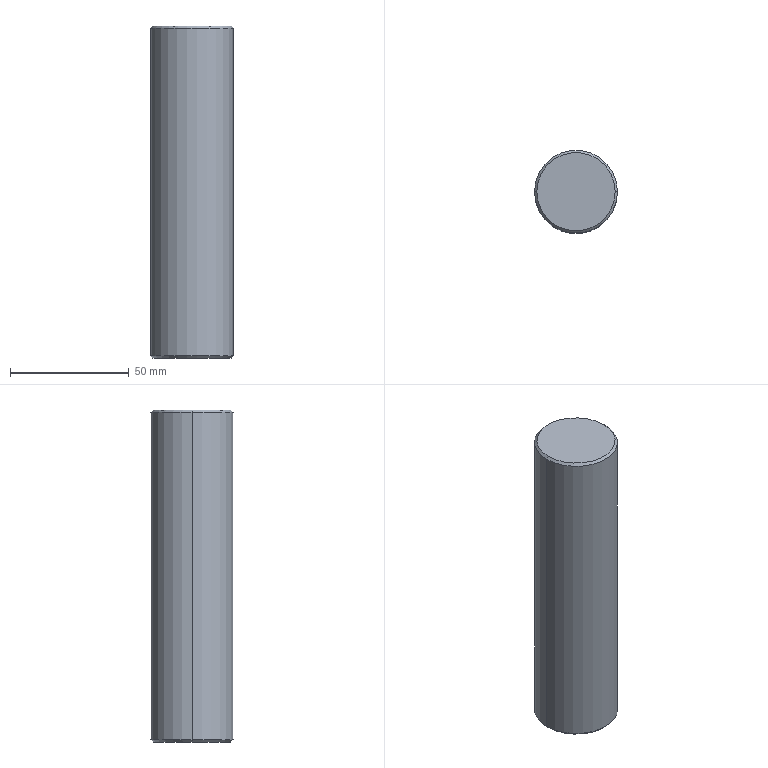Part | Creo | 1 solid | 16 faces | box 35 x 35 x 140 mm | volume 133063 mm3 | cone 8 | cylinder 6 | plane 2 | commonest cylinder face diameters 8.46 x2 10 x2 35 x2
STEP:
#1=CARTESIAN_POINT('',(0.,0.,0.));
#2=DIRECTION('',(0.,0.,1.));
#3=DIRECTION('',(1.,0.,0.));
#4=AXIS2_PLACEMENT_3D('',#1,#2,#3);
#5=CARTESIAN_POINT('',(16.5,43.,-260.5));
#6=VERTEX_POINT('',#5);
#7=CARTESIAN_POINT('',(-16.5,43.,-260.5));
#8=VERTEX_POINT('',#7);
#9=CARTESIAN_POINT('',(0.,43.,-260.5));
#10=DIRECTION('',(0.,0.,-1.));
#11=DIRECTION('',(1.,0.,0.));
#12=AXIS2_PLACEMENT_3D('',#9,#10,#11);
#13=CIRCLE('',#12,16.5);
#14=EDGE_CURVE('',#6,#8,#13,.T.);
#15=ORIENTED_EDGE('',*,*,#14,.F.);
#16=CARTESIAN_POINT('',(0.,43.,-260.5));
#17=DIRECTION('',(0.,0.,-1.));
#18=DIRECTION('',(-1.,0.,0.));
#19=AXIS2_PLACEMENT_3D('',#16,#17,#18);
#20=CIRCLE('',#19,16.5);
#21=EDGE_CURVE('',#8,#6,#20,.T.);
#22=ORIENTED_EDGE('',*,*,#21,.F.);
#23=EDGE_LOOP('',(#15,#22));
#24=FACE_OUTER_BOUND('',#23,.F.);
#25=CARTESIAN_POINT('',(-5.,43.,-260.5));
#26=VERTEX_POINT('',#25);
#27=CARTESIAN_POINT('',(5.,43.,-260.5));
#28=VERTEX_POINT('',#27);
#29=CARTESIAN_POINT('',(0.,43.,-260.5));
#30=DIRECTION('',(0.,0.,1.));
#31=DIRECTION('',(-1.,0.,0.));
#32=AXIS2_PLACEMENT_3D('',#29,#30,#31);
#33=CIRCLE('',#32,5.);
#34=EDGE_CURVE('',#26,#28,#33,.T.);
#35=ORIENTED_EDGE('',*,*,#34,.F.);
#36=CARTESIAN_POINT('',(0.,43.,-260.5));
#37=DIRECTION('',(0.,0.,1.));
#38=DIRECTION('',(1.,0.,0.));
#39=AXIS2_PLACEMENT_3D('',#36,#37,#38);
#40=CIRCLE('',#39,5.);
#41=EDGE_CURVE('',#28,#26,#40,.T.);
#42=ORIENTED_EDGE('',*,*,#41,.F.);
#43=EDGE_LOOP('',(#35,#42));
#44=FACE_BOUND('',#43,.F.);
#45=CARTESIAN_POINT('',(0.,43.,-260.5));
#46=DIRECTION('',(0.,0.,1.));
#47=DIRECTION('',(1.,0.,0.));
#48=AXIS2_PLACEMENT_3D('',#45,#46,#47);
#49=PLANE('',#48);
#50=ADVANCED_FACE('',(#24,#44),#49,.F.);
#51=ORIENTED_EDGE('',*,*,#14,.T.);
#52=CARTESIAN_POINT('',(-17.5,43.,-259.5));
#53=VERTEX_POINT('',#52);
#54=CARTESIAN_POINT('',(-16.5,43.,-260.5));
#55=DIRECTION('',(-0.7071,0.,0.7071));
#56=VECTOR('',#55,1.414);
#57=LINE('',#54,#56);
#58=EDGE_CURVE('',#8,#53,#57,.T.);
#59=ORIENTED_EDGE('',*,*,#58,.T.);
#60=CARTESIAN_POINT('',(17.5,43.,-259.5));
#61=VERTEX_POINT('',#60);
#62=CARTESIAN_POINT('',(0.,43.,-259.5));
#63=DIRECTION('',(0.,0.,-1.));
#64=DIRECTION('',(1.,0.,0.));
#65=AXIS2_PLACEMENT_3D('',#62,#63,#64);
#66=CIRCLE('',#65,17.5);
#67=EDGE_CURVE('',#61,#53,#66,.T.);
#68=ORIENTED_EDGE('',*,*,#67,.F.);
#69=CARTESIAN_POINT('',(16.5,43.,-260.5));
#70=DIRECTION('',(0.7071,0.,0.7071));
#71=VECTOR('',#70,1.414);
#72=LINE('',#69,#71);
#73=EDGE_CURVE('',#6,#61,#72,.T.);
#74=ORIENTED_EDGE('',*,*,#73,.F.);
#75=EDGE_LOOP('',(#51,#59,#68,#74));
#76=FACE_OUTER_BOUND('',#75,.F.);
#77=CARTESIAN_POINT('',(0.,43.,-260.));
#78=DIRECTION('',(0.,0.,1.));
#79=DIRECTION('',(1.,0.,0.));
#80=AXIS2_PLACEMENT_3D('',#77,#78,#79);
#81=CONICAL_SURFACE('',#80,17.,45.);
#82=ADVANCED_FACE('',(#76),#81,.T.);
#83=ORIENTED_EDGE('',*,*,#21,.T.);
#84=ORIENTED_EDGE('',*,*,#73,.T.);
#85=CARTESIAN_POINT('',(0.,43.,-259.5));
#86=DIRECTION('',(0.,0.,-1.));
#87=DIRECTION('',(-1.,0.,0.));
#88=AXIS2_PLACEMENT_3D('',#85,#86,#87);
#89=CIRCLE('',#88,17.5);
#90=EDGE_CURVE('',#53,#61,#89,.T.);
#91=ORIENTED_EDGE('',*,*,#90,.F.);
#92=ORIENTED_EDGE('',*,*,#58,.F.);
#93=EDGE_LOOP('',(#83,#84,#91,#92));
#94=FACE_OUTER_BOUND('',#93,.F.);
#95=CARTESIAN_POINT('',(0.,43.,-260.));
#96=DIRECTION('',(0.,0.,1.));
#97=DIRECTION('',(1.,0.,0.));
#98=AXIS2_PLACEMENT_3D('',#95,#96,#97);
#99=CONICAL_SURFACE('',#98,17.,45.);
#100=ADVANCED_FACE('',(#94),#99,.T.);
#101=ORIENTED_EDGE('',*,*,#90,.T.);
#102=CARTESIAN_POINT('',(17.5,43.,-121.5));
#103=VERTEX_POINT('',#102);
#104=CARTESIAN_POINT('',(17.5,43.,-121.5));
#105=DIRECTION('',(0.,0.,-1.));
#106=VECTOR('',#105,138.);
#107=LINE('',#104,#106);
#108=EDGE_CURVE('',#103,#61,#107,.T.);
#109=ORIENTED_EDGE('',*,*,#108,.F.);
#110=CARTESIAN_POINT('',(-17.5,43.,-121.5));
#111=VERTEX_POINT('',#110);
#112=CARTESIAN_POINT('',(0.,43.,-121.5));
#113=DIRECTION('',(0.,0.,1.));
#114=DIRECTION('',(1.,0.,0.));
#115=AXIS2_PLACEMENT_3D('',#112,#113,#114);
#116=CIRCLE('',#115,17.5);
#117=EDGE_CURVE('',#103,#111,#116,.T.);
#118=ORIENTED_EDGE('',*,*,#117,.T.);
#119=CARTESIAN_POINT('',(-17.5,43.,-121.5));
#120=DIRECTION('',(0.,0.,-1.));
#121=VECTOR('',#120,138.);
#122=LINE('',#119,#121);
#123=EDGE_CURVE('',#111,#53,#122,.T.);
#124=ORIENTED_EDGE('',*,*,#123,.T.);
#125=EDGE_LOOP('',(#101,#109,#118,#124));
#126=FACE_OUTER_BOUND('',#125,.F.);
#127=CARTESIAN_POINT('',(0.,43.,-120.5));
#128=DIRECTION('',(0.,0.,-1.));
#129=DIRECTION('',(-1.,0.,0.));
#130=AXIS2_PLACEMENT_3D('',#127,#128,#129);
#131=CYLINDRICAL_SURFACE('',#130,17.5);
#132=ADVANCED_FACE('',(#126),#131,.T.);
#133=ORIENTED_EDGE('',*,*,#67,.T.);
#134=ORIENTED_EDGE('',*,*,#123,.F.);
#135=CARTESIAN_POINT('',(0.,43.,-121.5));
#136=DIRECTION('',(0.,0.,1.));
#137=DIRECTION('',(-1.,0.,0.));
#138=AXIS2_PLACEMENT_3D('',#135,#136,#137);
#139=CIRCLE('',#138,17.5);
#140=EDGE_CURVE('',#111,#103,#139,.T.);
#141=ORIENTED_EDGE('',*,*,#140,.T.);
#142=ORIENTED_EDGE('',*,*,#108,.T.);
#143=EDGE_LOOP('',(#133,#134,#141,#142));
#144=FACE_OUTER_BOUND('',#143,.F.);
#145=CARTESIAN_POINT('',(0.,43.,-120.5));
#146=DIRECTION('',(0.,0.,-1.));
#147=DIRECTION('',(-1.,0.,0.));
#148=AXIS2_PLACEMENT_3D('',#145,#146,#147);
#149=CYLINDRICAL_SURFACE('',#148,17.5);
#150=ADVANCED_FACE('',(#144),#149,.T.);
#151=ORIENTED_EDGE('',*,*,#140,.F.);
#152=CARTESIAN_POINT('',(-16.5,43.,-120.5));
#153=VERTEX_POINT('',#152);
#154=CARTESIAN_POINT('',(-16.5,43.,-120.5));
#155=DIRECTION('',(-0.7071,0.,-0.7071));
#156=VECTOR('',#155,1.414);
#157=LINE('',#154,#156);
#158=EDGE_CURVE('',#153,#111,#157,.T.);
#159=ORIENTED_EDGE('',*,*,#158,.F.);
#160=CARTESIAN_POINT('',(16.5,43.,-120.5));
#161=VERTEX_POINT('',#160);
#162=CARTESIAN_POINT('',(0.,43.,-120.5));
#163=DIRECTION('',(0.,0.,1.));
#164=DIRECTION('',(-1.,0.,0.));
#165=AXIS2_PLACEMENT_3D('',#162,#163,#164);
#166=CIRCLE('',#165,16.5);
#167=EDGE_CURVE('',#153,#161,#166,.T.);
#168=ORIENTED_EDGE('',*,*,#167,.T.);
#169=CARTESIAN_POINT('',(16.5,43.,-120.5));
#170=DIRECTION('',(0.7071,0.,-0.7071));
#171=VECTOR('',#170,1.414);
#172=LINE('',#169,#171);
#173=EDGE_CURVE('',#161,#103,#172,.T.);
#174=ORIENTED_EDGE('',*,*,#173,.T.);
#175=EDGE_LOOP('',(#151,#159,#168,#174));
#176=FACE_OUTER_BOUND('',#175,.F.);
#177=CARTESIAN_POINT('',(0.,43.,-121.));
#178=DIRECTION('',(0.,0.,-1.));
#179=DIRECTION('',(-1.,0.,0.));
#180=AXIS2_PLACEMENT_3D('',#177,#178,#179);
#181=CONICAL_SURFACE('',#180,17.,45.);
#182=ADVANCED_FACE('',(#176),#181,.T.);
#183=ORIENTED_EDGE('',*,*,#117,.F.);
#184=ORIENTED_EDGE('',*,*,#173,.F.);
#185=CARTESIAN_POINT('',(0.,43.,-120.5));
#186=DIRECTION('',(0.,0.,1.));
#187=DIRECTION('',(1.,0.,0.));
#188=AXIS2_PLACEMENT_3D('',#185,#186,#187);
#189=CIRCLE('',#188,16.5);
#190=EDGE_CURVE('',#161,#153,#189,.T.);
#191=ORIENTED_EDGE('',*,*,#190,.T.);
#192=ORIENTED_EDGE('',*,*,#158,.T.);
#193=EDGE_LOOP('',(#183,#184,#191,#192));
#194=FACE_OUTER_BOUND('',#193,.F.);
#195=CARTESIAN_POINT('',(0.,43.,-121.));
#196=DIRECTION('',(0.,0.,-1.));
#197=DIRECTION('',(-1.,0.,0.));
#198=AXIS2_PLACEMENT_3D('',#195,#196,#197);
#199=CONICAL_SURFACE('',#198,17.,45.);
#200=ADVANCED_FACE('',(#194),#199,.T.);
#201=ORIENTED_EDGE('',*,*,#190,.F.);
#202=ORIENTED_EDGE('',*,*,#167,.F.);
#203=EDGE_LOOP('',(#201,#202));
#204=FACE_OUTER_BOUND('',#203,.F.);
#205=CARTESIAN_POINT('',(0.,43.,-120.5));
#206=DIRECTION('',(0.,0.,1.));
#207=DIRECTION('',(1.,0.,0.));
#208=AXIS2_PLACEMENT_3D('',#205,#206,#207);
#209=PLANE('',#208);
#210=ADVANCED_FACE('',(#204),#209,.T.);
#211=CARTESIAN_POINT('',(5.,43.,-244.5));
#212=VERTEX_POINT('',#211);
#213=CARTESIAN_POINT('',(-5.,43.,-244.5));
#214=VERTEX_POINT('',#213);
#215=CARTESIAN_POINT('',(0.,43.,-244.5));
#216=DIRECTION('',(0.,0.,-1.));
#217=DIRECTION('',(1.,0.,0.));
#218=AXIS2_PLACEMENT_3D('',#215,#216,#217);
#219=CIRCLE('',#218,5.);
#220=EDGE_CURVE('',#212,#214,#219,.T.);
#221=ORIENTED_EDGE('',*,*,#220,.T.);
#222=CARTESIAN_POINT('',(-5.,43.,-244.5));
#223=DIRECTION('',(0.,0.,-1.));
#224=VECTOR('',#223,16.);
#225=LINE('',#222,#224);
#226=EDGE_CURVE('',#214,#26,#225,.T.);
#227=ORIENTED_EDGE('',*,*,#226,.T.);
#228=ORIENTED_EDGE('',*,*,#34,.T.);
#229=CARTESIAN_POINT('',(5.,43.,-244.5));
#230=DIRECTION('',(0.,0.,-1.));
#231=VECTOR('',#230,16.);
#232=LINE('',#229,#231);
#233=EDGE_CURVE('',#212,#28,#232,.T.);
#234=ORIENTED_EDGE('',*,*,#233,.F.);
#235=EDGE_LOOP('',(#221,#227,#228,#234));
#236=FACE_OUTER_BOUND('',#235,.F.);
#237=CARTESIAN_POINT('',(0.,43.,-295.5));
#238=DIRECTION('',(0.,0.,-1.));
#239=DIRECTION('',(-1.,0.,0.));
#240=AXIS2_PLACEMENT_3D('',#237,#238,#239);
#241=CYLINDRICAL_SURFACE('',#240,5.);
#242=ADVANCED_FACE('',(#236),#241,.F.);
#243=CARTESIAN_POINT('',(-4.23,43.,-243.73));
#244=VERTEX_POINT('',#243);
#245=CARTESIAN_POINT('',(4.23,43.,-243.73));
#246=VERTEX_POINT('',#245);
#247=CARTESIAN_POINT('',(0.,43.,-243.73));
#248=DIRECTION('',(0.,0.,1.));
#249=DIRECTION('',(-1.,0.,0.));
#250=AXIS2_PLACEMENT_3D('',#247,#248,#249);
#251=CIRCLE('',#250,4.23);
#252=EDGE_CURVE('',#244,#246,#251,.T.);
#253=ORIENTED_EDGE('',*,*,#252,.F.);
#254=CARTESIAN_POINT('',(-4.23,43.,-243.73));
#255=DIRECTION('',(-0.7071,0.,-0.7071));
#256=VECTOR('',#255,1.089);
#257=LINE('',#254,#256);
#258=EDGE_CURVE('',#244,#214,#257,.T.);
#259=ORIENTED_EDGE('',*,*,#258,.T.);
#260=ORIENTED_EDGE('',*,*,#220,.F.);
#261=CARTESIAN_POINT('',(4.23,43.,-243.73));
#262=DIRECTION('',(0.7071,0.,-0.7071));
#263=VECTOR('',#262,1.089);
#264=LINE('',#261,#263);
#265=EDGE_CURVE('',#246,#212,#264,.T.);
#266=ORIENTED_EDGE('',*,*,#265,.F.);
#267=EDGE_LOOP('',(#253,#259,#260,#266));
#268=FACE_OUTER_BOUND('',#267,.F.);
#269=CARTESIAN_POINT('',(0.,43.,-244.115));
#270=DIRECTION('',(0.,0.,-1.));
#271=DIRECTION('',(-1.,0.,0.));
#272=AXIS2_PLACEMENT_3D('',#269,#270,#271);
#273=CONICAL_SURFACE('',#272,4.615,45.);
#274=ADVANCED_FACE('',(#268),#273,.F.);
#275=CARTESIAN_POINT('',(4.23,43.,-240.73));
#276=VERTEX_POINT('',#275);
#277=CARTESIAN_POINT('',(-4.23,43.,-240.73));
#278=VERTEX_POINT('',#277);
#279=CARTESIAN_POINT('',(0.,43.,-240.73));
#280=DIRECTION('',(0.,0.,-1.));
#281=DIRECTION('',(1.,0.,0.));
#282=AXIS2_PLACEMENT_3D('',#279,#280,#281);
#283=CIRCLE('',#282,4.23);
#284=EDGE_CURVE('',#276,#278,#283,.T.);
#285=ORIENTED_EDGE('',*,*,#284,.T.);
#286=CARTESIAN_POINT('',(-4.23,43.,-240.73));
#287=DIRECTION('',(0.,0.,-1.));
#288=VECTOR('',#287,3.);
#289=LINE('',#286,#288);
#290=EDGE_CURVE('',#278,#244,#289,.T.);
#291=ORIENTED_EDGE('',*,*,#290,.T.);
#292=ORIENTED_EDGE('',*,*,#252,.T.);
#293=CARTESIAN_POINT('',(4.23,43.,-240.73));
#294=DIRECTION('',(0.,0.,-1.));
#295=VECTOR('',#294,3.);
#296=LINE('',#293,#295);
#297=EDGE_CURVE('',#276,#246,#296,.T.);
#298=ORIENTED_EDGE('',*,*,#297,.F.);
#299=EDGE_LOOP('',(#285,#291,#292,#298));
#300=FACE_OUTER_BOUND('',#299,.F.);
#301=CARTESIAN_POINT('',(0.,43.,-295.5));
#302=DIRECTION('',(0.,0.,-1.));
#303=DIRECTION('',(-1.,0.,0.));
#304=AXIS2_PLACEMENT_3D('',#301,#302,#303);
#305=CYLINDRICAL_SURFACE('',#304,4.23);
#306=ADVANCED_FACE('',(#300),#305,.F.);
#307=ORIENTED_EDGE('',*,*,#284,.F.);
#308=CARTESIAN_POINT('',(0.,43.,-238.188));
#309=VERTEX_POINT('',#308);
#310=CARTESIAN_POINT('',(0.,43.,-238.188));
#311=DIRECTION('',(0.8572,0.,-0.515));
#312=VECTOR('',#311,4.935);
#313=LINE('',#310,#312);
#314=EDGE_CURVE('',#309,#276,#313,.T.);
#315=ORIENTED_EDGE('',*,*,#314,.F.);
#316=CARTESIAN_POINT('',(0.,43.,-238.188));
#317=DIRECTION('',(-0.8572,0.,-0.515));
#318=VECTOR('',#317,4.935);
#319=LINE('',#316,#318);
#320=EDGE_CURVE('',#309,#278,#319,.T.);
#321=ORIENTED_EDGE('',*,*,#320,.T.);
#322=EDGE_LOOP('',(#307,#315,#321));
#323=FACE_OUTER_BOUND('',#322,.F.);
#324=CARTESIAN_POINT('',(0.,43.,-239.505));
#325=DIRECTION('',(0.,0.,-1.));
#326=DIRECTION('',(-1.,0.,0.));
#327=AXIS2_PLACEMENT_3D('',#324,#325,#326);
#328=CONICAL_SURFACE('',#327,2.191,59.);
#329=ADVANCED_FACE('',(#323),#328,.F.);
#330=CARTESIAN_POINT('',(0.,43.,-240.73));
#331=DIRECTION('',(0.,0.,-1.));
#332=DIRECTION('',(-1.,0.,0.));
#333=AXIS2_PLACEMENT_3D('',#330,#331,#332);
#334=CIRCLE('',#333,4.23);
#335=EDGE_CURVE('',#278,#276,#334,.T.);
#336=ORIENTED_EDGE('',*,*,#335,.F.);
#337=ORIENTED_EDGE('',*,*,#320,.F.);
#338=ORIENTED_EDGE('',*,*,#314,.T.);
#339=EDGE_LOOP('',(#336,#337,#338));
#340=FACE_OUTER_BOUND('',#339,.F.);
#341=CARTESIAN_POINT('',(0.,43.,-239.505));
#342=DIRECTION('',(0.,0.,-1.));
#343=DIRECTION('',(-1.,0.,0.));
#344=AXIS2_PLACEMENT_3D('',#341,#342,#343);
#345=CONICAL_SURFACE('',#344,2.191,59.);
#346=ADVANCED_FACE('',(#340),#345,.F.);
#347=ORIENTED_EDGE('',*,*,#335,.T.);
#348=ORIENTED_EDGE('',*,*,#297,.T.);
#349=CARTESIAN_POINT('',(0.,43.,-243.73));
#350=DIRECTION('',(0.,0.,1.));
#351=DIRECTION('',(1.,0.,0.));
#352=AXIS2_PLACEMENT_3D('',#349,#350,#351);
#353=CIRCLE('',#352,4.23);
#354=EDGE_CURVE('',#246,#244,#353,.T.);
#355=ORIENTED_EDGE('',*,*,#354,.T.);
#356=ORIENTED_EDGE('',*,*,#290,.F.);
#357=EDGE_LOOP('',(#347,#348,#355,#356));
#358=FACE_OUTER_BOUND('',#357,.F.);
#359=CARTESIAN_POINT('',(0.,43.,-295.5));
#360=DIRECTION('',(0.,0.,-1.));
#361=DIRECTION('',(-1.,0.,0.));
#362=AXIS2_PLACEMENT_3D('',#359,#360,#361);
#363=CYLINDRICAL_SURFACE('',#362,4.23);
#364=ADVANCED_FACE('',(#358),#363,.F.);
#365=ORIENTED_EDGE('',*,*,#354,.F.);
#366=ORIENTED_EDGE('',*,*,#265,.T.);
#367=CARTESIAN_POINT('',(0.,43.,-244.5));
#368=DIRECTION('',(0.,0.,-1.));
#369=DIRECTION('',(-1.,0.,0.));
#370=AXIS2_PLACEMENT_3D('',#367,#368,#369);
#371=CIRCLE('',#370,5.);
#372=EDGE_CURVE('',#214,#212,#371,.T.);
#373=ORIENTED_EDGE('',*,*,#372,.F.);
#374=ORIENTED_EDGE('',*,*,#258,.F.);
#375=EDGE_LOOP('',(#365,#366,#373,#374));
#376=FACE_OUTER_BOUND('',#375,.F.);
#377=CARTESIAN_POINT('',(0.,43.,-244.115));
#378=DIRECTION('',(0.,0.,-1.));
#379=DIRECTION('',(-1.,0.,0.));
#380=AXIS2_PLACEMENT_3D('',#377,#378,#379);
#381=CONICAL_SURFACE('',#380,4.615,45.);
#382=ADVANCED_FACE('',(#376),#381,.F.);
#383=ORIENTED_EDGE('',*,*,#372,.T.);
#384=ORIENTED_EDGE('',*,*,#233,.T.);
#385=ORIENTED_EDGE('',*,*,#41,.T.);
#386=ORIENTED_EDGE('',*,*,#226,.F.);
#387=EDGE_LOOP('',(#383,#384,#385,#386));
#388=FACE_OUTER_BOUND('',#387,.F.);
#389=CARTESIAN_POINT('',(0.,43.,-295.5));
#390=DIRECTION('',(0.,0.,-1.));
#391=DIRECTION('',(-1.,0.,0.));
#392=AXIS2_PLACEMENT_3D('',#389,#390,#391);
#393=CYLINDRICAL_SURFACE('',#392,5.);
#394=ADVANCED_FACE('',(#388),#393,.F.);
#395=CLOSED_SHELL('',(#50,#82,#100,#132,#150,#182,#200,#210,#242,#274,#306,#329,#346,#364,#382,#394));
#396=MANIFOLD_SOLID_BREP('',#395);
#397=(LENGTH_UNIT()NAMED_UNIT(*)SI_UNIT(.MILLI.,.METRE.));
#398=UNCERTAINTY_MEASURE_WITH_UNIT(LENGTH_MEASURE(0.01485),#397,'','');
#399=(NAMED_UNIT(*)PLANE_ANGLE_UNIT()SI_UNIT($,.RADIAN.));
#400=PLANE_ANGLE_MEASURE_WITH_UNIT(PLANE_ANGLE_MEASURE(0.01745),#399);
#401=(CONVERSION_BASED_UNIT('DEGREE',#400)NAMED_UNIT(*)PLANE_ANGLE_UNIT());
#402=(NAMED_UNIT(*)SI_UNIT($,.STERADIAN.)SOLID_ANGLE_UNIT());
#403=(GEOMETRIC_REPRESENTATION_CONTEXT(3)GLOBAL_UNCERTAINTY_ASSIGNED_CONTEXT((#398))GLOBAL_UNIT_ASSIGNED_CONTEXT((#397,#401,#402))REPRESENTATION_CONTEXT('',''));
#404=ADVANCED_BREP_SHAPE_REPRESENTATION('',(#4,#396),#403);